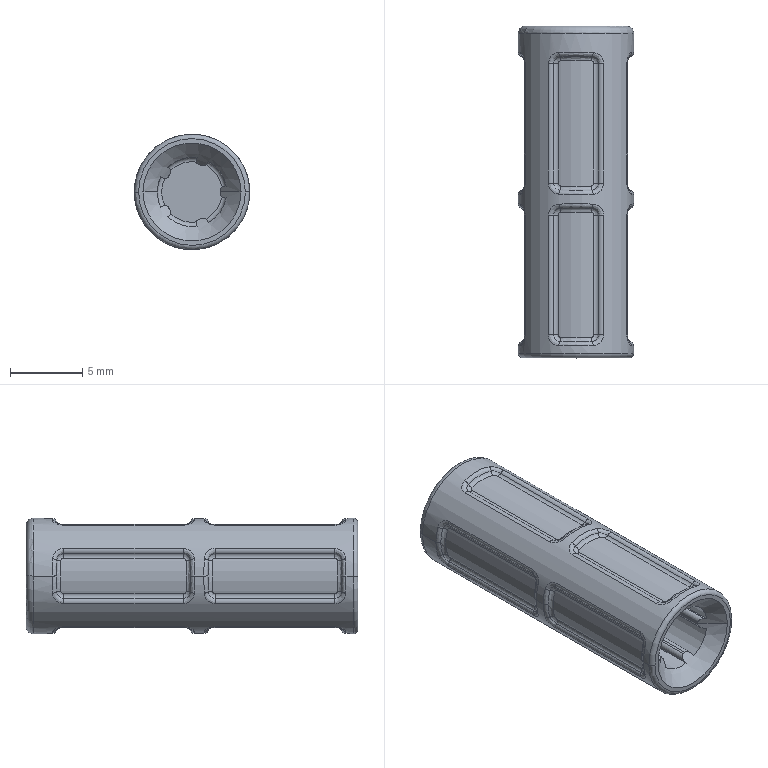Part | STEP file | ZXW735-L-228_2_1_1 | 1 solid | 190 faces | box 8 x 23 x 8 mm | volume 701.957 mm3 | spline 104 | cylinder 62 | plane 13 | torus 9 | cone 2 | commonest cylinder face diameters 0.6 x42 7.2 x8 3.9 x5 4.8 x5 8 x2